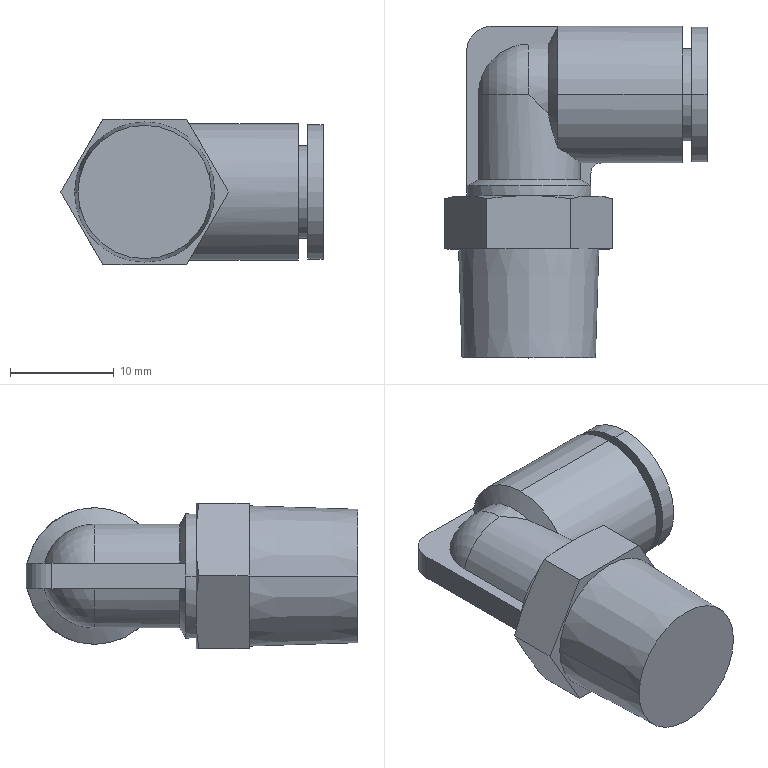Part | SolidWorks | features BaseBody 1 | 1 solid | 56 faces | box 25.283 x 32 x 14 mm | volume 4555 mm3 | plane 26 | cylinder 16 | cone 12 | sphere 2 | commonest cylinder face diameters 10 x4 8 x2 8.95 x2 12 x2 13 x2 13.18 x2